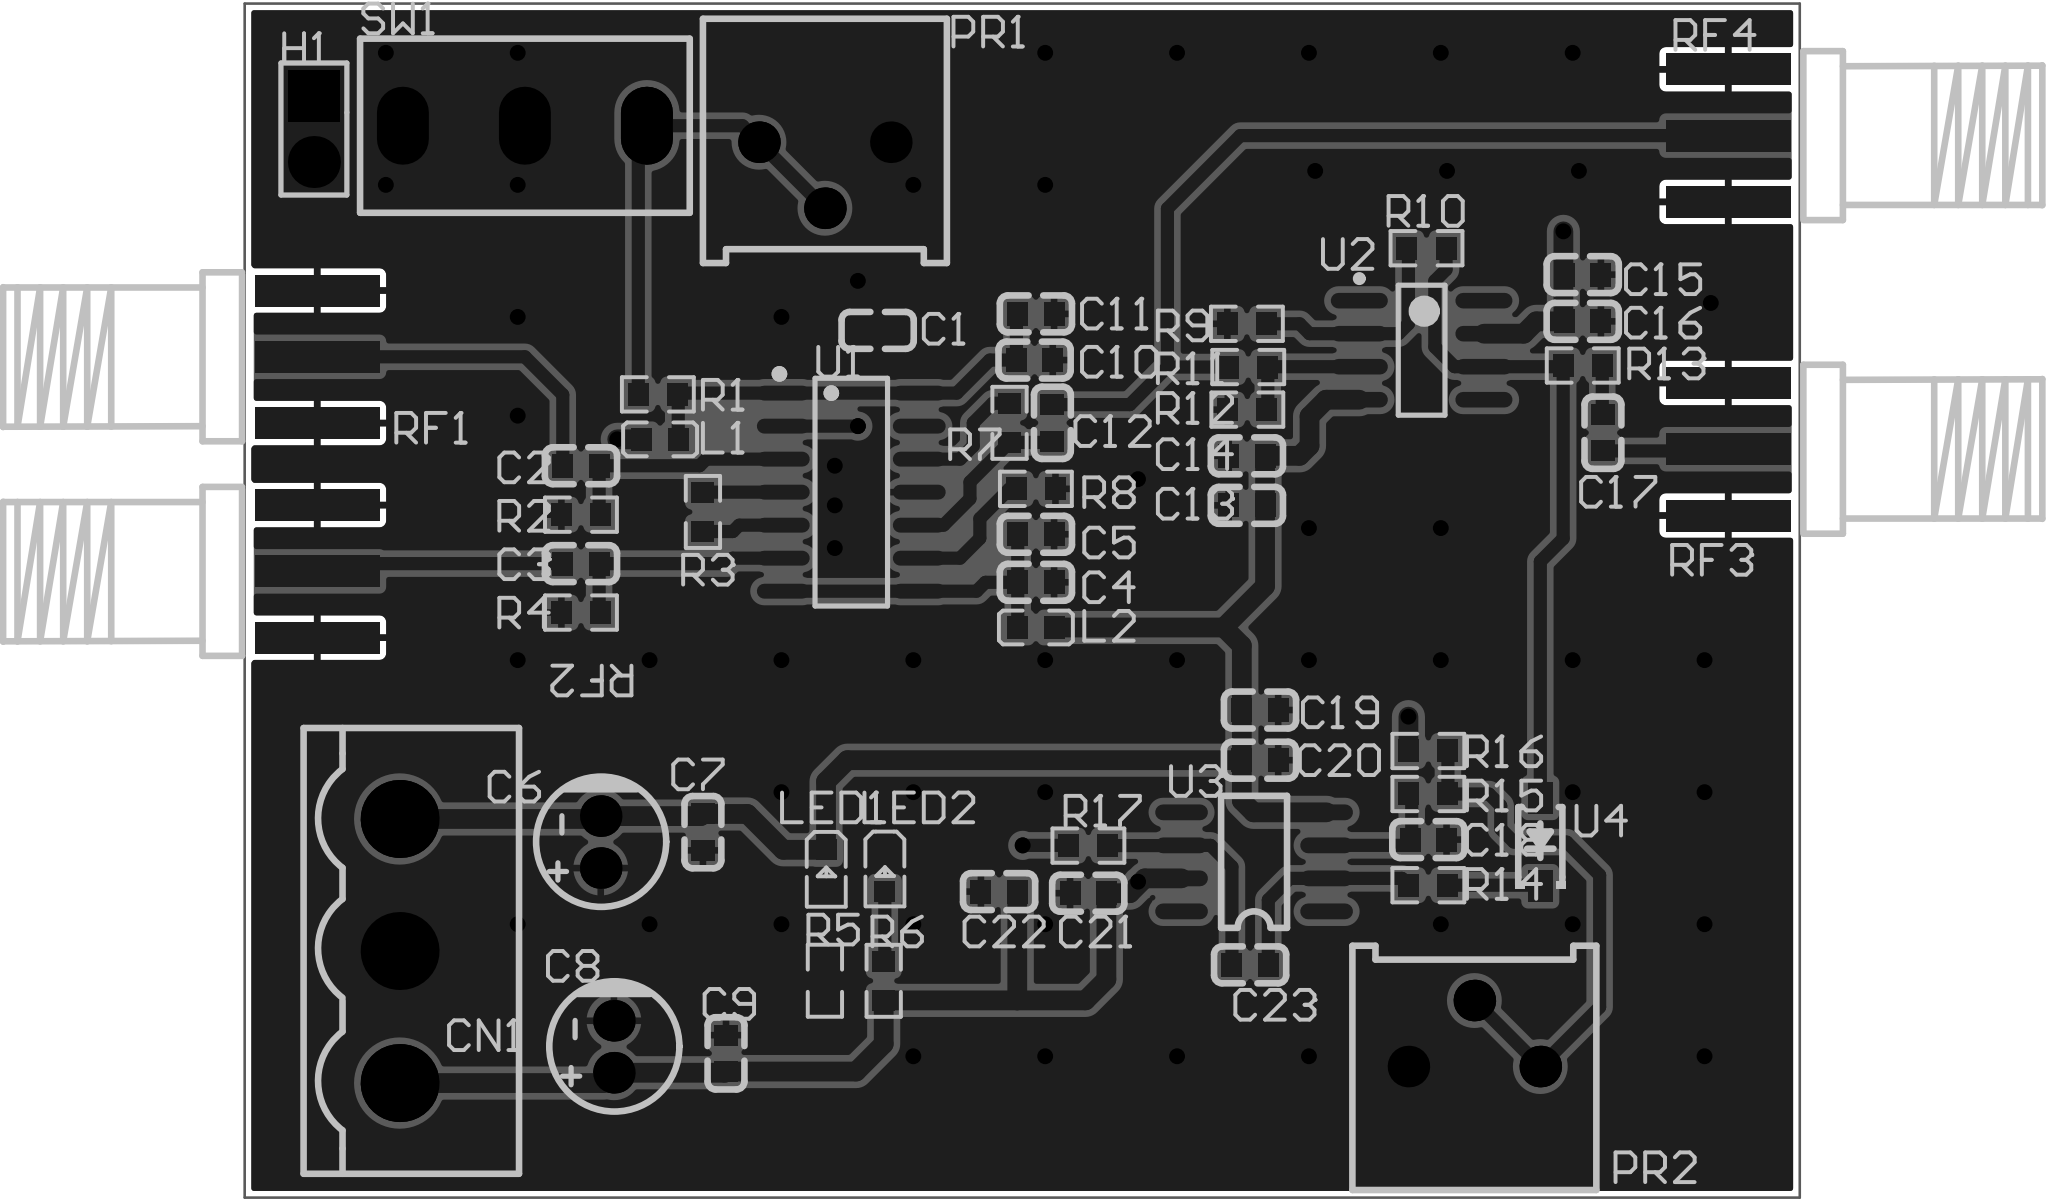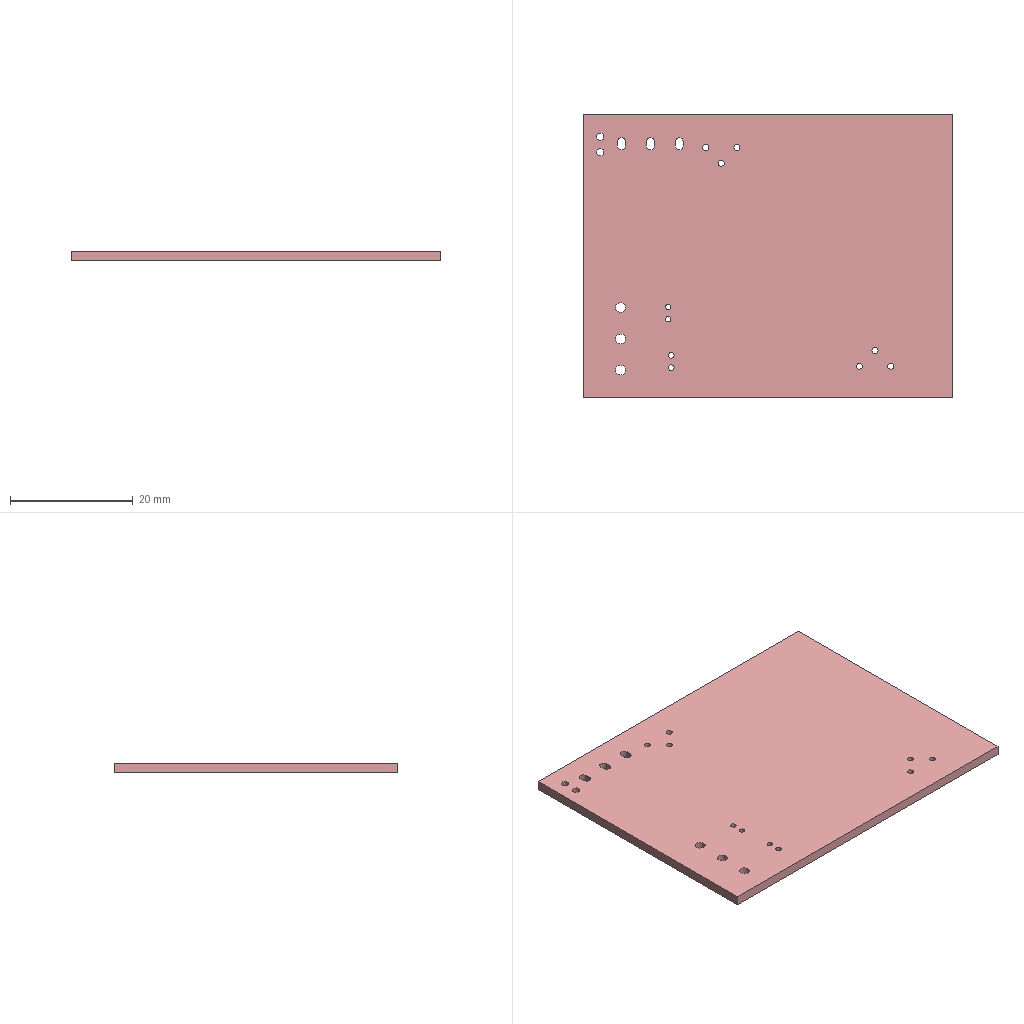Circuit board layout | Altium Designer | box 59.9 x 45.9 x 1.6 mm
Layer stack:
# Altium Designer layer stack of  (unit mm; dielectric type: 0 none, 1 core, 2 prepreg, 3 surface material)
index,name,kind,layer,copper_thickness_mm,dielectric_type,dielectric_thickness_mm,dielectric_material,dielectric_constant
0,Top Paste Mask Layer,other,,,,,,
1,Top Silkscreen Layer,other,,,,,,
2,Top Solder Mask Layer,dielectric,,,3,0.01,,3.3
3,Top Layer,copper,Top Layer,0.035,,,,
4,Dielectric 1,dielectric,,,3,1.51,FR4,4.5
5,Bottom Layer,copper,Bottom Layer,0.035,,,,
6,Bottom Solder Mask Layer,dielectric,,,3,0.01,,3.3
7,Bottom Silkscreen Layer,other,,,,,,
8,Bottom Paste Mask Layer,other,,,,,,
# drill layer pairs: low layer,high layer
drill_pair,Top Layer,Bottom Layer
Part placement:
Designator,Comment,Layer,Footprint,Center-X(mm),Center-Y(mm),Rotation
C1,100nF,TopLayer,C0603,110.01,109.563,180
C2,100nF,TopLayer,C0603,98.58,104.356,0
C3,100nF,TopLayer,C0603,98.58,100.59,0
C4,100nF,TopLayer,C0603,116.106,99.871,0
C5,1uF,TopLayer,C0603,116.106,101.719,180
C6,10uF,TopLayer,CAP-TH_BD5.0-P2.00-D0.5-FD-A,99.342,89.878,90
C7,100nF,TopLayer,C0603,103.279,90.259,90
C8,10uF,TopLayer,CAP-TH_BD5.0-P2.00-D0.5-FD-A,99.85,82.004,90
C9,100nF,TopLayer,C0603,104.168,81.75,270
C10,1uF,TopLayer,C0603,116.055,108.421,0
C11,100nF,TopLayer,C0603,116.106,110.198,0
C12,100nF,TopLayer,C0603,116.741,106.007,90
C13,100nF,TopLayer,C0603,124.234,102.832,0
C14,1uF,TopLayer,C0603,124.234,104.737,0
C15,1uF,TopLayer,C0603,137.172,111.709,0
C16,100nF,TopLayer,C0603,137.172,109.91,0
C17,100nF,TopLayer,C0603,137.95,105.626,270
C18,100nF,TopLayer,C0603,131.225,89.973,180
C19,100nF,TopLayer,C0603,124.739,94.958,180
C20,1uF,TopLayer,C0603,124.739,93.028,180
C21,100nF,TopLayer,C0603,118.122,87.911,180
C22,1uF,TopLayer,C0603,114.688,87.973,180
C23,100nF,TopLayer,C0603,124.358,85.154,180
L1,10uH,TopLayer,L0603,101.628,105.372,0
L2,10uH,TopLayer,L0603,116.106,98.133,180
LED1,,TopLayer,LED_0603,108.024,88.781,270
LED2,,TopLayer,LED_0603,110.284,88.793,270
PR1,10K,TopLayer,R_3386P,107.978,115.532,90
PR2,10K,TopLayer,R_3386P,132.997,82.512,270
R1,10K,TopLayer,R0603,101.543,107.101,180
R2,51R,TopLayer,R0603,98.58,102.473,180
R3,10,TopLayer,R0603,103.279,102.578,90
R4,50R,TopLayer,R0603,98.58,98.707,0
R5,1K,TopLayer,R0603,107.978,84.544,90
R6,1K,TopLayer,R0603,110.243,84.54,90
R7,1K,TopLayer,R0603,115.09,106.007,270
R8,0,TopLayer,R0603,116.106,103.467,180
R9,51R,TopLayer,R0603,124.234,109.817,0
R10,1K,TopLayer,R0603,131.153,112.725,0
R11,10R,TopLayer,R0603,124.286,108.153,0
R12,51R,TopLayer,R0603,124.251,106.515,0
R13,10R,TopLayer,R0603,137.172,108.213,0
R14,1K,TopLayer,R0603,131.225,88.218,0
R15,100,TopLayer,R0603,131.225,91.728,0
R16,3K,TopLayer,R0603,131.225,93.382,180
R17,100,TopLayer,R0603,118.129,89.742,0
SW1,SS-12D10L5,TopLayer,SW-TH_SS-12D10L5,96.421,117.437,180
U1,VCA821ID,TopLayer,SOIC-14_L8.7-W3.9-P1.27-LS6.0-BL,108.994,103.34,270
U2,OPA695,TopLayer,SOIC-8,130.965,108.801,0
U3,OPA820,TopLayer,SOP8,124.511,89.117,180
U4,1N4150,TopLayer,SOD-123_L2.7-W1.6-LS3.7-RD-1,135.537,89.878,90
H1,PZ254V-11-02P,TopLayer,HDR-TH_2P-P2.54-V-M,88.293,117.31,270
CN1,WJ2EDGVC-5.08-03P-14-00A,TopLayer,CONN-TH_3P-P5.08-WJ2EDGVC-3P,91.595,85.687,270
RF1,6GHz,TopLayer,SMA-SMD_BWSMA-KE-P001,88.42,108.547,180
RF2,6GHz,TopLayer,SMA-SMD_BWSMA-KE-P001,88.42,100.292,180
RF3,6GHz,TopLayer,SMA-SMD_BWSMA-KE-P001,142.776,104.991,0
RF4,6GHz,TopLayer,SMA-SMD_BWSMA-KE-P001,142.776,117.056,0
Pad and via stacks:
# Altium Designer via and pad stacks of  (unit mm). Each distinct definition once, with the count of objects using it.
# via: kind,start_layer,end_layer,hole_mm,diameter_mm,mode(0 simple;1 top-mid-bottom;2 full stack),diameter_per_layer,count,example_net
# pad: kind,layer,hole_mm,hole_type(0 round;1 square;2 slot),plating,top_size,top_shape(1 round;2 rect;3 octagon;9 rounded rect),mid_size,bottom_size,mode,footprint,size_per_layer,count,example
pad,Top Layer,0,0,plated,0.8x0.9,2,0.8x0.9,0.8x0.9,0,C0603,,42,C1.2
pad,Top Layer,0,0,plated,0.8x0.864,2,0.8x0.864,0.8x0.864,0,L0603,,4,L1.1
pad,Top Layer,0,0,plated,0.8001x0.8001,2,0.8001x0.8001,0.8001x0.8001,0,LED_0603,,4,LED1.1
pad,Top Layer,0,0,plated,0.8065x0.864,2,0.8065x0.864,0.8065x0.864,0,R0603,,34,R1.2
pad,Top Layer,0,0,plated,0.574x2.038,1,0.574x2.038,0.574x2.038,0,SOIC-14_L8.7-W3.9-P1.27-LS6.0-BL,,14,U1.8
pad,Top Layer,0,0,plated,0.6x2.2,1,0.6x2.2,0.6x2.2,0,SOIC-8,,8,U2.1
pad,Top Layer,0,0,plated,2.032x0.6096,1,2.032x0.6096,2.032x0.6096,0,SOP8,,8,U3.3
pad,Top Layer,0,0,plated,1.2x0.95,2,1.2x0.95,1.2x0.95,0,SOD-123_L2.7-W1.6-LS3.7-RD-1,,2,U4.2
pad,Top Layer,0,0,plated,4.8x1.2,2,4.8x1.2,4.8x1.2,0,SMA-SMD_BWSMA-KE-P001,,12,RF1.1
pad,Multi-Layer,0.9,0,plated,1.6x1.6,1,1.6x1.6,1.6x1.6,0,CAP-TH_BD5.0-P2.00-D0.5-FD-A,,4,C6.2
pad,Multi-Layer,1.001,0,plated,1.6x1.6,1,1.6x1.6,1.6x1.6,0,R_3386P,,6,PR1.2
pad,Multi-Layer,1.3,2,plated,2x3,1,2x3,2x3,0,SW-TH_SS-12D10L5,,3,SW1.1
pad,Multi-Layer,1.2,0,plated,2x2,2,2x2,2x2,0,HDR-TH_2P-P2.54-V-M,,1,H1.1
pad,Multi-Layer,1.2,0,plated,2x2,1,2x2,2x2,0,HDR-TH_2P-P2.54-V-M,,1,H1.2
pad,Multi-Layer,1.6,0,plated,3x3,1,3x3,3x3,0,CONN-TH_3P-P5.08-WJ2EDGVC-3P,,3,CN1.1
pad,Bottom Layer,0,0,plated,4.8x1.2,2,4.8x1.2,4.8x1.2,0,SMA-SMD_BWSMA-KE-P001,,8,RF1.3
via,Top Layer,Bottom Layer,0.3048,0.61,0,,59,VG
Copper pours:
name,layer,net,type(0 solid;1 hatched;2 none)
Top Layer-GND,Top Layer,GND,0
Bottom Layer-GND,Bottom Layer,GND,0